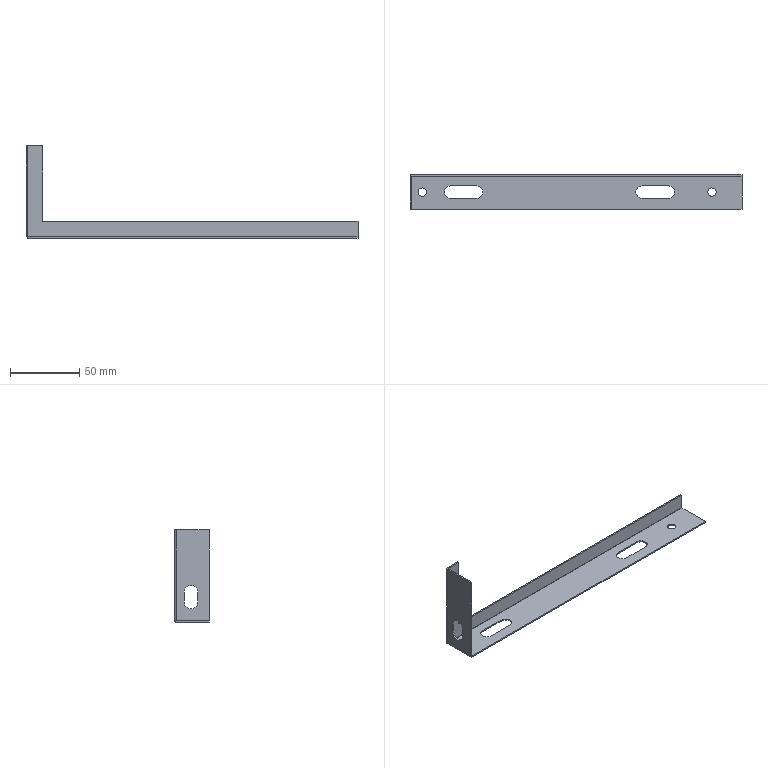Part | 1 solid | 40 faces | box 240 x 25 x 66.7 mm | volume 10129 mm3 | plane 26 | cylinder 14 | commonest cylinder face diameters 6 x4 9 x4 0.4 x2 2.4 x2 10 x2
STEP:
#1=CARTESIAN_POINT('',(97.7,-15.5,-0.2));
#2=VERTEX_POINT('',#1);
#3=CARTESIAN_POINT('',(97.7,-9.5,-0.2));
#4=VERTEX_POINT('',#3);
#5=CARTESIAN_POINT('',(97.7,-12.5,-0.2));
#6=DIRECTION('',(0.,0.,-1.));
#7=DIRECTION('',(0.,1.,0.));
#8=AXIS2_PLACEMENT_3D('',#5,#6,#7);
#9=CIRCLE('',#8,3.);
#10=EDGE_CURVE('',#2,#4,#9,.T.);
#11=ORIENTED_EDGE('',*,*,#10,.F.);
#12=CARTESIAN_POINT('',(97.7,-15.5,-1.2));
#13=VERTEX_POINT('',#12);
#14=CARTESIAN_POINT('',(97.7,-15.5,8.8));
#15=DIRECTION('',(0.,0.,-1.));
#16=VECTOR('',#15,1000.);
#17=LINE('',#14,#16);
#18=EDGE_CURVE('',#2,#13,#17,.T.);
#19=ORIENTED_EDGE('',*,*,#18,.T.);
#20=CARTESIAN_POINT('',(97.7,-9.5,-1.2));
#21=VERTEX_POINT('',#20);
#22=CARTESIAN_POINT('',(97.7,-12.5,-1.2));
#23=DIRECTION('',(0.,0.,-1.));
#24=DIRECTION('',(0.,1.,0.));
#25=AXIS2_PLACEMENT_3D('',#22,#23,#24);
#26=CIRCLE('',#25,3.);
#27=EDGE_CURVE('',#13,#21,#26,.T.);
#28=ORIENTED_EDGE('',*,*,#27,.T.);
#29=CARTESIAN_POINT('',(97.7,-9.5,8.8));
#30=DIRECTION('',(0.,0.,-1.));
#31=VECTOR('',#30,1000.);
#32=LINE('',#29,#31);
#33=EDGE_CURVE('',#4,#21,#32,.T.);
#34=ORIENTED_EDGE('',*,*,#33,.F.);
#35=EDGE_LOOP('',(#11,#19,#28,#34));
#36=FACE_OUTER_BOUND('',#35,.T.);
#37=CARTESIAN_POINT('',(97.7,-12.5,8.8));
#38=DIRECTION('',(0.,0.,-1.));
#39=DIRECTION('',(0.,1.,0.));
#40=AXIS2_PLACEMENT_3D('',#37,#38,#39);
#41=CYLINDRICAL_SURFACE('',#40,3.);
#42=ADVANCED_FACE('',(#36),#41,.F.);
#43=CARTESIAN_POINT('',(-111.8,-15.5,-0.2));
#44=VERTEX_POINT('',#43);
#45=CARTESIAN_POINT('',(-111.8,-9.5,-0.2));
#46=VERTEX_POINT('',#45);
#47=CARTESIAN_POINT('',(-111.8,-12.5,-0.2));
#48=DIRECTION('',(0.,0.,-1.));
#49=DIRECTION('',(0.,1.,0.));
#50=AXIS2_PLACEMENT_3D('',#47,#48,#49);
#51=CIRCLE('',#50,3.);
#52=EDGE_CURVE('',#44,#46,#51,.T.);
#53=ORIENTED_EDGE('',*,*,#52,.F.);
#54=CARTESIAN_POINT('',(-111.8,-15.5,-1.2));
#55=VERTEX_POINT('',#54);
#56=CARTESIAN_POINT('',(-111.8,-15.5,8.8));
#57=DIRECTION('',(0.,0.,-1.));
#58=VECTOR('',#57,1000.);
#59=LINE('',#56,#58);
#60=EDGE_CURVE('',#44,#55,#59,.T.);
#61=ORIENTED_EDGE('',*,*,#60,.T.);
#62=CARTESIAN_POINT('',(-111.8,-9.5,-1.2));
#63=VERTEX_POINT('',#62);
#64=CARTESIAN_POINT('',(-111.8,-12.5,-1.2));
#65=DIRECTION('',(0.,0.,-1.));
#66=DIRECTION('',(0.,1.,0.));
#67=AXIS2_PLACEMENT_3D('',#64,#65,#66);
#68=CIRCLE('',#67,3.);
#69=EDGE_CURVE('',#55,#63,#68,.T.);
#70=ORIENTED_EDGE('',*,*,#69,.T.);
#71=CARTESIAN_POINT('',(-111.8,-9.5,8.8));
#72=DIRECTION('',(0.,0.,-1.));
#73=VECTOR('',#72,1000.);
#74=LINE('',#71,#73);
#75=EDGE_CURVE('',#46,#63,#74,.T.);
#76=ORIENTED_EDGE('',*,*,#75,.F.);
#77=EDGE_LOOP('',(#53,#61,#70,#76));
#78=FACE_OUTER_BOUND('',#77,.T.);
#79=CARTESIAN_POINT('',(-111.8,-12.5,8.8));
#80=DIRECTION('',(0.,0.,-1.));
#81=DIRECTION('',(0.,1.,0.));
#82=AXIS2_PLACEMENT_3D('',#79,#80,#81);
#83=CYLINDRICAL_SURFACE('',#82,3.);
#84=ADVANCED_FACE('',(#78),#83,.F.);
#85=CARTESIAN_POINT('',(119.4,-1.,11.));
#86=VERTEX_POINT('',#85);
#87=CARTESIAN_POINT('',(-108.4,-1.,11.));
#88=VERTEX_POINT('',#87);
#89=CARTESIAN_POINT('',(-119.4,-1.,11.));
#90=DIRECTION('',(-1.,0.,0.));
#91=VECTOR('',#90,1000.);
#92=LINE('',#89,#91);
#93=EDGE_CURVE('',#86,#88,#92,.T.);
#94=ORIENTED_EDGE('',*,*,#93,.T.);
#95=CARTESIAN_POINT('',(-108.4,-1.,65.5));
#96=VERTEX_POINT('',#95);
#97=CARTESIAN_POINT('',(-108.4,-1.,65.5));
#98=DIRECTION('',(0.,0.,1.));
#99=VECTOR('',#98,1000.);
#100=LINE('',#97,#99);
#101=EDGE_CURVE('',#88,#96,#100,.T.);
#102=ORIENTED_EDGE('',*,*,#101,.T.);
#103=CARTESIAN_POINT('',(-119.4,-1.,65.5));
#104=VERTEX_POINT('',#103);
#105=CARTESIAN_POINT('',(-119.4,-1.,65.5));
#106=DIRECTION('',(1.,0.,0.));
#107=VECTOR('',#106,1000.);
#108=LINE('',#105,#107);
#109=EDGE_CURVE('',#104,#96,#108,.T.);
#110=ORIENTED_EDGE('',*,*,#109,.F.);
#111=CARTESIAN_POINT('',(-119.4,-1.,0.));
#112=VERTEX_POINT('',#111);
#113=CARTESIAN_POINT('',(-119.4,-1.,65.5));
#114=DIRECTION('',(0.,0.,-1.));
#115=VECTOR('',#114,1000.);
#116=LINE('',#113,#115);
#117=EDGE_CURVE('',#104,#112,#116,.T.);
#118=ORIENTED_EDGE('',*,*,#117,.T.);
#119=CARTESIAN_POINT('',(119.4,-1.,0.));
#120=VERTEX_POINT('',#119);
#121=CARTESIAN_POINT('',(-119.4,-1.,0.));
#122=DIRECTION('',(1.,0.,0.));
#123=VECTOR('',#122,1000.);
#124=LINE('',#121,#123);
#125=EDGE_CURVE('',#112,#120,#124,.T.);
#126=ORIENTED_EDGE('',*,*,#125,.T.);
#127=CARTESIAN_POINT('',(119.4,-1.,65.5));
#128=DIRECTION('',(0.,0.,-1.));
#129=VECTOR('',#128,1000.);
#130=LINE('',#127,#129);
#131=EDGE_CURVE('',#86,#120,#130,.T.);
#132=ORIENTED_EDGE('',*,*,#131,.F.);
#133=EDGE_LOOP('',(#94,#102,#110,#118,#126,#132));
#134=FACE_OUTER_BOUND('',#133,.T.);
#135=CARTESIAN_POINT('',(-119.4,-1.,65.5));
#136=DIRECTION('',(0.,1.,0.));
#137=DIRECTION('',(-1.,0.,0.));
#138=AXIS2_PLACEMENT_3D('',#135,#136,#137);
#139=PLANE('',#138);
#140=ADVANCED_FACE('',(#134),#139,.F.);
#141=CARTESIAN_POINT('',(119.4,0.,11.));
#142=VERTEX_POINT('',#141);
#143=CARTESIAN_POINT('',(119.4,-10.,11.));
#144=DIRECTION('',(0.,1.,0.));
#145=VECTOR('',#144,1000.);
#146=LINE('',#143,#145);
#147=EDGE_CURVE('',#86,#142,#146,.T.);
#148=ORIENTED_EDGE('',*,*,#147,.F.);
#149=ORIENTED_EDGE('',*,*,#131,.T.);
#150=CARTESIAN_POINT('',(119.4,0.,0.));
#151=VERTEX_POINT('',#150);
#152=CARTESIAN_POINT('',(119.4,0.,0.));
#153=DIRECTION('',(0.,-1.,0.));
#154=VECTOR('',#153,1000.);
#155=LINE('',#152,#154);
#156=EDGE_CURVE('',#151,#120,#155,.T.);
#157=ORIENTED_EDGE('',*,*,#156,.F.);
#158=CARTESIAN_POINT('',(119.4,0.,65.5));
#159=DIRECTION('',(0.,0.,-1.));
#160=VECTOR('',#159,1000.);
#161=LINE('',#158,#160);
#162=EDGE_CURVE('',#142,#151,#161,.T.);
#163=ORIENTED_EDGE('',*,*,#162,.F.);
#164=EDGE_LOOP('',(#148,#149,#157,#163));
#165=FACE_OUTER_BOUND('',#164,.T.);
#166=CARTESIAN_POINT('',(119.4,0.,65.5));
#167=DIRECTION('',(1.,0.,0.));
#168=DIRECTION('',(0.,0.,-1.));
#169=AXIS2_PLACEMENT_3D('',#166,#167,#168);
#170=PLANE('',#169);
#171=ADVANCED_FACE('',(#165),#170,.T.);
#172=CARTESIAN_POINT('',(-108.4,0.,11.));
#173=VERTEX_POINT('',#172);
#174=CARTESIAN_POINT('',(-108.4,0.,65.5));
#175=VERTEX_POINT('',#174);
#176=CARTESIAN_POINT('',(-108.4,0.,65.5));
#177=DIRECTION('',(0.,0.,1.));
#178=VECTOR('',#177,1000.);
#179=LINE('',#176,#178);
#180=EDGE_CURVE('',#173,#175,#179,.T.);
#181=ORIENTED_EDGE('',*,*,#180,.F.);
#182=CARTESIAN_POINT('',(119.4,0.,11.));
#183=DIRECTION('',(-1.,0.,0.));
#184=VECTOR('',#183,1000.);
#185=LINE('',#182,#184);
#186=EDGE_CURVE('',#142,#173,#185,.T.);
#187=ORIENTED_EDGE('',*,*,#186,.F.);
#188=ORIENTED_EDGE('',*,*,#162,.T.);
#189=CARTESIAN_POINT('',(-119.4,0.,0.));
#190=VERTEX_POINT('',#189);
#191=CARTESIAN_POINT('',(-119.4,0.,0.));
#192=DIRECTION('',(1.,0.,0.));
#193=VECTOR('',#192,1000.);
#194=LINE('',#191,#193);
#195=EDGE_CURVE('',#190,#151,#194,.T.);
#196=ORIENTED_EDGE('',*,*,#195,.F.);
#197=CARTESIAN_POINT('',(-119.4,0.,65.5));
#198=VERTEX_POINT('',#197);
#199=CARTESIAN_POINT('',(-119.4,0.,65.5));
#200=DIRECTION('',(0.,0.,-1.));
#201=VECTOR('',#200,1000.);
#202=LINE('',#199,#201);
#203=EDGE_CURVE('',#198,#190,#202,.T.);
#204=ORIENTED_EDGE('',*,*,#203,.F.);
#205=CARTESIAN_POINT('',(-119.4,0.,65.5));
#206=DIRECTION('',(1.,0.,0.));
#207=VECTOR('',#206,1000.);
#208=LINE('',#205,#207);
#209=EDGE_CURVE('',#198,#175,#208,.T.);
#210=ORIENTED_EDGE('',*,*,#209,.T.);
#211=EDGE_LOOP('',(#181,#187,#188,#196,#204,#210));
#212=FACE_OUTER_BOUND('',#211,.T.);
#213=CARTESIAN_POINT('',(-119.4,0.,65.5));
#214=DIRECTION('',(0.,1.,0.));
#215=DIRECTION('',(-1.,0.,0.));
#216=AXIS2_PLACEMENT_3D('',#213,#214,#215);
#217=PLANE('',#216);
#218=ADVANCED_FACE('',(#212),#217,.T.);
#219=ORIENTED_EDGE('',*,*,#109,.T.);
#220=CARTESIAN_POINT('',(-108.4,0.,65.5));
#221=DIRECTION('',(0.,1.,0.));
#222=VECTOR('',#221,1000.);
#223=LINE('',#220,#222);
#224=EDGE_CURVE('',#96,#175,#223,.T.);
#225=ORIENTED_EDGE('',*,*,#224,.T.);
#226=ORIENTED_EDGE('',*,*,#209,.F.);
#227=CARTESIAN_POINT('',(-119.4,-1.,65.5));
#228=DIRECTION('',(0.,1.,0.));
#229=VECTOR('',#228,1000.);
#230=LINE('',#227,#229);
#231=EDGE_CURVE('',#104,#198,#230,.T.);
#232=ORIENTED_EDGE('',*,*,#231,.F.);
#233=EDGE_LOOP('',(#219,#225,#226,#232));
#234=FACE_OUTER_BOUND('',#233,.T.);
#235=CARTESIAN_POINT('',(0.,0.,65.5));
#236=DIRECTION('',(0.,0.,-1.));
#237=DIRECTION('',(-1.,0.,0.));
#238=AXIS2_PLACEMENT_3D('',#235,#236,#237);
#239=PLANE('',#238);
#240=ADVANCED_FACE('',(#234),#239,.F.);
#241=ORIENTED_EDGE('',*,*,#147,.T.);
#242=ORIENTED_EDGE('',*,*,#186,.T.);
#243=CARTESIAN_POINT('',(-108.4,-10.,11.));
#244=DIRECTION('',(0.,1.,0.));
#245=VECTOR('',#244,1000.);
#246=LINE('',#243,#245);
#247=EDGE_CURVE('',#88,#173,#246,.T.);
#248=ORIENTED_EDGE('',*,*,#247,.F.);
#249=ORIENTED_EDGE('',*,*,#93,.F.);
#250=EDGE_LOOP('',(#241,#242,#248,#249));
#251=FACE_OUTER_BOUND('',#250,.T.);
#252=CARTESIAN_POINT('',(119.4,-10.,11.));
#253=DIRECTION('',(0.,0.,-1.));
#254=DIRECTION('',(-1.,0.,0.));
#255=AXIS2_PLACEMENT_3D('',#252,#253,#254);
#256=PLANE('',#255);
#257=ADVANCED_FACE('',(#251),#256,.F.);
#258=ORIENTED_EDGE('',*,*,#247,.T.);
#259=ORIENTED_EDGE('',*,*,#180,.T.);
#260=ORIENTED_EDGE('',*,*,#224,.F.);
#261=ORIENTED_EDGE('',*,*,#101,.F.);
#262=EDGE_LOOP('',(#258,#259,#260,#261));
#263=FACE_OUTER_BOUND('',#262,.T.);
#264=CARTESIAN_POINT('',(-108.4,-10.,65.5));
#265=DIRECTION('',(-1.,0.,0.));
#266=DIRECTION('',(0.,0.,1.));
#267=AXIS2_PLACEMENT_3D('',#264,#265,#266);
#268=PLANE('',#267);
#269=ADVANCED_FACE('',(#263),#268,.F.);
#270=CARTESIAN_POINT('',(-119.4,-1.2,-0.2));
#271=VERTEX_POINT('',#270);
#272=CARTESIAN_POINT('',(-119.4,-1.2,-1.2));
#273=VERTEX_POINT('',#272);
#274=CARTESIAN_POINT('',(-119.4,-1.2,-1.2));
#275=DIRECTION('',(0.,0.,-1.));
#276=VECTOR('',#275,1000.);
#277=LINE('',#274,#276);
#278=EDGE_CURVE('',#271,#273,#277,.T.);
#279=ORIENTED_EDGE('',*,*,#278,.F.);
#280=CARTESIAN_POINT('',(-119.4,-1.2,0.));
#281=DIRECTION('',(-1.,0.,0.));
#282=DIRECTION('',(0.,1.,0.));
#283=AXIS2_PLACEMENT_3D('',#280,#281,#282);
#284=CIRCLE('',#283,0.2);
#285=EDGE_CURVE('',#112,#271,#284,.T.);
#286=ORIENTED_EDGE('',*,*,#285,.F.);
#287=CARTESIAN_POINT('',(-119.4,-1.,0.));
#288=DIRECTION('',(0.,1.,0.));
#289=VECTOR('',#288,1000.);
#290=LINE('',#287,#289);
#291=EDGE_CURVE('',#112,#190,#290,.T.);
#292=ORIENTED_EDGE('',*,*,#291,.T.);
#293=CARTESIAN_POINT('',(-119.4,-1.2,0.));
#294=DIRECTION('',(-1.,0.,0.));
#295=DIRECTION('',(0.,1.,0.));
#296=AXIS2_PLACEMENT_3D('',#293,#294,#295);
#297=CIRCLE('',#296,1.2);
#298=EDGE_CURVE('',#190,#273,#297,.T.);
#299=ORIENTED_EDGE('',*,*,#298,.T.);
#300=EDGE_LOOP('',(#279,#286,#292,#299));
#301=FACE_OUTER_BOUND('',#300,.T.);
#302=CARTESIAN_POINT('',(-119.4,-1.2,0.));
#303=DIRECTION('',(-1.,0.,0.));
#304=DIRECTION('',(0.,-1.,0.));
#305=AXIS2_PLACEMENT_3D('',#302,#303,#304);
#306=PLANE('',#305);
#307=ADVANCED_FACE('',(#301),#306,.T.);
#308=CARTESIAN_POINT('',(119.4,-1.2,-0.2));
#309=VERTEX_POINT('',#308);
#310=CARTESIAN_POINT('',(119.4,-1.2,0.));
#311=DIRECTION('',(1.,0.,0.));
#312=DIRECTION('',(0.,1.,0.));
#313=AXIS2_PLACEMENT_3D('',#310,#311,#312);
#314=CIRCLE('',#313,0.2);
#315=EDGE_CURVE('',#309,#120,#314,.T.);
#316=ORIENTED_EDGE('',*,*,#315,.F.);
#317=CARTESIAN_POINT('',(119.4,-1.2,-1.2));
#318=VERTEX_POINT('',#317);
#319=CARTESIAN_POINT('',(119.4,-1.2,-0.2));
#320=DIRECTION('',(0.,0.,-1.));
#321=VECTOR('',#320,1000.);
#322=LINE('',#319,#321);
#323=EDGE_CURVE('',#309,#318,#322,.T.);
#324=ORIENTED_EDGE('',*,*,#323,.T.);
#325=CARTESIAN_POINT('',(119.4,-1.2,0.));
#326=DIRECTION('',(1.,0.,0.));
#327=DIRECTION('',(0.,1.,0.));
#328=AXIS2_PLACEMENT_3D('',#325,#326,#327);
#329=CIRCLE('',#328,1.2);
#330=EDGE_CURVE('',#318,#151,#329,.T.);
#331=ORIENTED_EDGE('',*,*,#330,.T.);
#332=ORIENTED_EDGE('',*,*,#156,.T.);
#333=EDGE_LOOP('',(#316,#324,#331,#332));
#334=FACE_OUTER_BOUND('',#333,.T.);
#335=CARTESIAN_POINT('',(119.4,-1.2,0.));
#336=DIRECTION('',(-1.,0.,0.));
#337=DIRECTION('',(0.,-1.,0.));
#338=AXIS2_PLACEMENT_3D('',#335,#336,#337);
#339=PLANE('',#338);
#340=ADVANCED_FACE('',(#334),#339,.F.);
#341=ORIENTED_EDGE('',*,*,#195,.T.);
#342=ORIENTED_EDGE('',*,*,#330,.F.);
#343=CARTESIAN_POINT('',(0.,-1.2,-1.2));
#344=DIRECTION('',(1.,0.,0.));
#345=VECTOR('',#344,1000.);
#346=LINE('',#343,#345);
#347=EDGE_CURVE('',#273,#318,#346,.T.);
#348=ORIENTED_EDGE('',*,*,#347,.F.);
#349=ORIENTED_EDGE('',*,*,#298,.F.);
#350=EDGE_LOOP('',(#341,#342,#348,#349));
#351=FACE_OUTER_BOUND('',#350,.T.);
#352=CARTESIAN_POINT('',(119.4,-1.2,0.));
#353=DIRECTION('',(1.,0.,0.));
#354=DIRECTION('',(0.,0.,-1.));
#355=AXIS2_PLACEMENT_3D('',#352,#353,#354);
#356=CYLINDRICAL_SURFACE('',#355,1.2);
#357=ADVANCED_FACE('',(#351),#356,.T.);
#358=ORIENTED_EDGE('',*,*,#125,.F.);
#359=ORIENTED_EDGE('',*,*,#285,.T.);
#360=CARTESIAN_POINT('',(-119.4,-1.2,-0.2));
#361=DIRECTION('',(1.,0.,0.));
#362=VECTOR('',#361,1000.);
#363=LINE('',#360,#362);
#364=EDGE_CURVE('',#271,#309,#363,.T.);
#365=ORIENTED_EDGE('',*,*,#364,.T.);
#366=ORIENTED_EDGE('',*,*,#315,.T.);
#367=EDGE_LOOP('',(#358,#359,#365,#366));
#368=FACE_OUTER_BOUND('',#367,.T.);
#369=CARTESIAN_POINT('',(119.4,-1.2,0.));
#370=DIRECTION('',(1.,0.,0.));
#371=DIRECTION('',(0.,0.,-1.));
#372=AXIS2_PLACEMENT_3D('',#369,#370,#371);
#373=CYLINDRICAL_SURFACE('',#372,0.2);
#374=ADVANCED_FACE('',(#368),#373,.F.);
#375=CARTESIAN_POINT('',(119.4,-25.,-1.2));
#376=VERTEX_POINT('',#375);
#377=CARTESIAN_POINT('',(119.4,-1.,-1.2));
#378=DIRECTION('',(0.,1.,0.));
#379=VECTOR('',#378,1000.);
#380=LINE('',#377,#379);
#381=EDGE_CURVE('',#376,#318,#380,.T.);
#382=ORIENTED_EDGE('',*,*,#381,.T.);
#383=ORIENTED_EDGE('',*,*,#323,.F.);
#384=CARTESIAN_POINT('',(119.4,-25.,-0.2));
#385=VERTEX_POINT('',#384);
#386=CARTESIAN_POINT('',(119.4,0.,-0.2));
#387=DIRECTION('',(0.,1.,0.));
#388=VECTOR('',#387,1000.);
#389=LINE('',#386,#388);
#390=EDGE_CURVE('',#385,#309,#389,.T.);
#391=ORIENTED_EDGE('',*,*,#390,.F.);
#392=CARTESIAN_POINT('',(119.4,-25.,-1.2));
#393=DIRECTION('',(0.,0.,1.));
#394=VECTOR('',#393,1000.);
#395=LINE('',#392,#394);
#396=EDGE_CURVE('',#376,#385,#395,.T.);
#397=ORIENTED_EDGE('',*,*,#396,.F.);
#398=EDGE_LOOP('',(#382,#383,#391,#397));
#399=FACE_OUTER_BOUND('',#398,.T.);
#400=CARTESIAN_POINT('',(119.4,-1.,-1.2));
#401=DIRECTION('',(1.,0.,0.));
#402=DIRECTION('',(0.,0.,-1.));
#403=AXIS2_PLACEMENT_3D('',#400,#401,#402);
#404=PLANE('',#403);
#405=ADVANCED_FACE('',(#399),#404,.T.);
#406=CARTESIAN_POINT('',(-119.4,-25.,-0.2));
#407=VERTEX_POINT('',#406);
#408=CARTESIAN_POINT('',(-119.4,0.,-0.2));
#409=DIRECTION('',(0.,-1.,0.));
#410=VECTOR('',#409,1000.);
#411=LINE('',#408,#410);
#412=EDGE_CURVE('',#271,#407,#411,.T.);
#413=ORIENTED_EDGE('',*,*,#412,.F.);
#414=ORIENTED_EDGE('',*,*,#278,.T.);
#415=CARTESIAN_POINT('',(-119.4,-25.,-1.2));
#416=VERTEX_POINT('',#415);
#417=CARTESIAN_POINT('',(-119.4,-25.,-1.2));
#418=DIRECTION('',(0.,-1.,0.));
#419=VECTOR('',#418,1000.);
#420=LINE('',#417,#419);
#421=EDGE_CURVE('',#273,#416,#420,.T.);
#422=ORIENTED_EDGE('',*,*,#421,.T.);
#423=CARTESIAN_POINT('',(-119.4,-25.,-1.2));
#424=DIRECTION('',(0.,0.,1.));
#425=VECTOR('',#424,1000.);
#426=LINE('',#423,#425);
#427=EDGE_CURVE('',#416,#407,#426,.T.);
#428=ORIENTED_EDGE('',*,*,#427,.T.);
#429=EDGE_LOOP('',(#413,#414,#422,#428));
#430=FACE_OUTER_BOUND('',#429,.T.);
#431=CARTESIAN_POINT('',(-119.4,-25.,-1.2));
#432=DIRECTION('',(-1.,0.,0.));
#433=DIRECTION('',(0.,0.,1.));
#434=AXIS2_PLACEMENT_3D('',#431,#432,#433);
#435=PLANE('',#434);
#436=ADVANCED_FACE('',(#430),#435,.T.);
#437=CARTESIAN_POINT('',(97.7,-12.5,-1.2));
#438=DIRECTION('',(0.,0.,-1.));
#439=DIRECTION('',(0.,1.,0.));
#440=AXIS2_PLACEMENT_3D('',#437,#438,#439);
#441=CIRCLE('',#440,3.);
#442=EDGE_CURVE('',#21,#13,#441,.T.);
#443=ORIENTED_EDGE('',*,*,#442,.F.);
#444=ORIENTED_EDGE('',*,*,#27,.F.);
#445=EDGE_LOOP('',(#443,#444));
#446=FACE_BOUND('',#445,.T.);
#447=CARTESIAN_POINT('',(-111.8,-12.5,-1.2));
#448=DIRECTION('',(0.,0.,-1.));
#449=DIRECTION('',(0.,1.,0.));
#450=AXIS2_PLACEMENT_3D('',#447,#448,#449);
#451=CIRCLE('',#450,3.);
#452=EDGE_CURVE('',#63,#55,#451,.T.);
#453=ORIENTED_EDGE('',*,*,#452,.F.);
#454=ORIENTED_EDGE('',*,*,#69,.F.);
#455=EDGE_LOOP('',(#453,#454));
#456=FACE_BOUND('',#455,.T.);
#457=CARTESIAN_POINT('',(47.2,-17.,-1.2));
#458=VERTEX_POINT('',#457);
#459=CARTESIAN_POINT('',(47.2,-8.,-1.2));
#460=VERTEX_POINT('',#459);
#461=CARTESIAN_POINT('',(47.2,-12.5,-1.2));
#462=DIRECTION('',(0.,0.,-1.));
#463=DIRECTION('',(0.,1.,0.));
#464=AXIS2_PLACEMENT_3D('',#461,#462,#463);
#465=CIRCLE('',#464,4.5);
#466=EDGE_CURVE('',#458,#460,#465,.T.);
#467=ORIENTED_EDGE('',*,*,#466,.F.);
#468=CARTESIAN_POINT('',(66.2,-17.,-1.2));
#469=VERTEX_POINT('',#468);
#470=CARTESIAN_POINT('',(47.2,-17.,-1.2));
#471=DIRECTION('',(-1.,0.,0.));
#472=VECTOR('',#471,1000.);
#473=LINE('',#470,#472);
#474=EDGE_CURVE('',#469,#458,#473,.T.);
#475=ORIENTED_EDGE('',*,*,#474,.F.);
#476=CARTESIAN_POINT('',(66.2,-8.,-1.2));
#477=VERTEX_POINT('',#476);
#478=CARTESIAN_POINT('',(66.2,-12.5,-1.2));
#479=DIRECTION('',(0.,0.,-1.));
#480=DIRECTION('',(0.,1.,0.));
#481=AXIS2_PLACEMENT_3D('',#478,#479,#480);
#482=CIRCLE('',#481,4.5);
#483=EDGE_CURVE('',#477,#469,#482,.T.);
#484=ORIENTED_EDGE('',*,*,#483,.F.);
#485=CARTESIAN_POINT('',(47.2,-8.,-1.2));
#486=DIRECTION('',(1.,0.,0.));
#487=VECTOR('',#486,1000.);
#488=LINE('',#485,#487);
#489=EDGE_CURVE('',#460,#477,#488,.T.);
#490=ORIENTED_EDGE('',*,*,#489,.F.);
#491=EDGE_LOOP('',(#467,#475,#484,#490));
#492=FACE_BOUND('',#491,.T.);
#493=CARTESIAN_POINT('',(-91.3,-17.,-1.2));
#494=VERTEX_POINT('',#493);
#495=CARTESIAN_POINT('',(-91.3,-8.,-1.2));
#496=VERTEX_POINT('',#495);
#497=CARTESIAN_POINT('',(-91.3,-12.5,-1.2));
#498=DIRECTION('',(0.,0.,-1.));
#499=DIRECTION('',(0.,1.,0.));
#500=AXIS2_PLACEMENT_3D('',#497,#498,#499);
#501=CIRCLE('',#500,4.5);
#502=EDGE_CURVE('',#494,#496,#501,.T.);
#503=ORIENTED_EDGE('',*,*,#502,.F.);
#504=CARTESIAN_POINT('',(-72.3,-17.,-1.2));
#505=VERTEX_POINT('',#504);
#506=CARTESIAN_POINT('',(-91.3,-17.,-1.2));
#507=DIRECTION('',(-1.,0.,0.));
#508=VECTOR('',#507,1000.);
#509=LINE('',#506,#508);
#510=EDGE_CURVE('',#505,#494,#509,.T.);
#511=ORIENTED_EDGE('',*,*,#510,.F.);
#512=CARTESIAN_POINT('',(-72.3,-8.,-1.2));
#513=VERTEX_POINT('',#512);
#514=CARTESIAN_POINT('',(-72.3,-12.5,-1.2));
#515=DIRECTION('',(0.,0.,-1.));
#516=DIRECTION('',(0.,1.,0.));
#517=AXIS2_PLACEMENT_3D('',#514,#515,#516);
#518=CIRCLE('',#517,4.5);
#519=EDGE_CURVE('',#513,#505,#518,.T.);
#520=ORIENTED_EDGE('',*,*,#519,.F.);
#521=CARTESIAN_POINT('',(-91.3,-8.,-1.2));
#522=DIRECTION('',(1.,0.,0.));
#523=VECTOR('',#522,1000.);
#524=LINE('',#521,#523);
#525=EDGE_CURVE('',#496,#513,#524,.T.);
#526=ORIENTED_EDGE('',*,*,#525,.F.);
#527=EDGE_LOOP('',(#503,#511,#520,#526));
#528=FACE_BOUND('',#527,.T.);
#529=ORIENTED_EDGE('',*,*,#421,.F.);
#530=ORIENTED_EDGE('',*,*,#347,.T.);
#531=ORIENTED_EDGE('',*,*,#381,.F.);
#532=CARTESIAN_POINT('',(119.4,-25.,-1.2));
#533=DIRECTION('',(1.,0.,0.));
#534=VECTOR('',#533,1000.);
#535=LINE('',#532,#534);
#536=EDGE_CURVE('',#416,#376,#535,.T.);
#537=ORIENTED_EDGE('',*,*,#536,.F.);
#538=EDGE_LOOP('',(#529,#530,#531,#537));
#539=FACE_OUTER_BOUND('',#538,.T.);
#540=CARTESIAN_POINT('',(0.,0.,-1.2));
#541=DIRECTION('',(0.,0.,-1.));
#542=DIRECTION('',(0.,1.,0.));
#543=AXIS2_PLACEMENT_3D('',#540,#541,#542);
#544=PLANE('',#543);
#545=ADVANCED_FACE('',(#446,#456,#492,#528,#539),#544,.T.);
#546=CARTESIAN_POINT('',(97.7,-12.5,-0.2));
#547=DIRECTION('',(0.,0.,-1.));
#548=DIRECTION('',(0.,1.,0.));
#549=AXIS2_PLACEMENT_3D('',#546,#547,#548);
#550=CIRCLE('',#549,3.);
#551=EDGE_CURVE('',#4,#2,#550,.T.);
#552=ORIENTED_EDGE('',*,*,#551,.T.);
#553=ORIENTED_EDGE('',*,*,#10,.T.);
#554=EDGE_LOOP('',(#552,#553));
#555=FACE_BOUND('',#554,.T.);
#556=CARTESIAN_POINT('',(-111.8,-12.5,-0.2));
#557=DIRECTION('',(0.,0.,-1.));
#558=DIRECTION('',(0.,1.,0.));
#559=AXIS2_PLACEMENT_3D('',#556,#557,#558);
#560=CIRCLE('',#559,3.);
#561=EDGE_CURVE('',#46,#44,#560,.T.);
#562=ORIENTED_EDGE('',*,*,#561,.T.);
#563=ORIENTED_EDGE('',*,*,#52,.T.);
#564=EDGE_LOOP('',(#562,#563));
#565=FACE_BOUND('',#564,.T.);
#566=CARTESIAN_POINT('',(66.2,-17.,-0.2));
#567=VERTEX_POINT('',#566);
#568=CARTESIAN_POINT('',(47.2,-17.,-0.2));
#569=VERTEX_POINT('',#568);
#570=CARTESIAN_POINT('',(0.,-17.,-0.2));
#571=DIRECTION('',(-1.,0.,0.));
#572=VECTOR('',#571,1000.);
#573=LINE('',#570,#572);
#574=EDGE_CURVE('',#567,#569,#573,.T.);
#575=ORIENTED_EDGE('',*,*,#574,.T.);
#576=CARTESIAN_POINT('',(47.2,-8.,-0.2));
#577=VERTEX_POINT('',#576);
#578=CARTESIAN_POINT('',(47.2,-12.5,-0.2));
#579=DIRECTION('',(0.,0.,-1.));
#580=DIRECTION('',(0.,1.,0.));
#581=AXIS2_PLACEMENT_3D('',#578,#579,#580);
#582=CIRCLE('',#581,4.5);
#583=EDGE_CURVE('',#569,#577,#582,.T.);
#584=ORIENTED_EDGE('',*,*,#583,.T.);
#585=CARTESIAN_POINT('',(66.2,-8.,-0.2));
#586=VERTEX_POINT('',#585);
#587=CARTESIAN_POINT('',(0.,-8.,-0.2));
#588=DIRECTION('',(1.,0.,0.));
#589=VECTOR('',#588,1000.);
#590=LINE('',#587,#589);
#591=EDGE_CURVE('',#577,#586,#590,.T.);
#592=ORIENTED_EDGE('',*,*,#591,.T.);
#593=CARTESIAN_POINT('',(66.2,-12.5,-0.2));
#594=DIRECTION('',(0.,0.,-1.));
#595=DIRECTION('',(0.,1.,0.));
#596=AXIS2_PLACEMENT_3D('',#593,#594,#595);
#597=CIRCLE('',#596,4.5);
#598=EDGE_CURVE('',#586,#567,#597,.T.);
#599=ORIENTED_EDGE('',*,*,#598,.T.);
#600=EDGE_LOOP('',(#575,#584,#592,#599));
#601=FACE_BOUND('',#600,.T.);
#602=CARTESIAN_POINT('',(-72.3,-17.,-0.2));
#603=VERTEX_POINT('',#602);
#604=CARTESIAN_POINT('',(-91.3,-17.,-0.2));
#605=VERTEX_POINT('',#604);
#606=CARTESIAN_POINT('',(0.,-17.,-0.2));
#607=DIRECTION('',(-1.,0.,0.));
#608=VECTOR('',#607,1000.);
#609=LINE('',#606,#608);
#610=EDGE_CURVE('',#603,#605,#609,.T.);
#611=ORIENTED_EDGE('',*,*,#610,.T.);
#612=CARTESIAN_POINT('',(-91.3,-8.,-0.2));
#613=VERTEX_POINT('',#612);
#614=CARTESIAN_POINT('',(-91.3,-12.5,-0.2));
#615=DIRECTION('',(0.,0.,-1.));
#616=DIRECTION('',(0.,1.,0.));
#617=AXIS2_PLACEMENT_3D('',#614,#615,#616);
#618=CIRCLE('',#617,4.5);
#619=EDGE_CURVE('',#605,#613,#618,.T.);
#620=ORIENTED_EDGE('',*,*,#619,.T.);
#621=CARTESIAN_POINT('',(-72.3,-8.,-0.2));
#622=VERTEX_POINT('',#621);
#623=CARTESIAN_POINT('',(0.,-8.,-0.2));
#624=DIRECTION('',(1.,0.,0.));
#625=VECTOR('',#624,1000.);
#626=LINE('',#623,#625);
#627=EDGE_CURVE('',#613,#622,#626,.T.);
#628=ORIENTED_EDGE('',*,*,#627,.T.);
#629=CARTESIAN_POINT('',(-72.3,-12.5,-0.2));
#630=DIRECTION('',(0.,0.,-1.));
#631=DIRECTION('',(0.,1.,0.));
#632=AXIS2_PLACEMENT_3D('',#629,#630,#631);
#633=CIRCLE('',#632,4.5);
#634=EDGE_CURVE('',#622,#603,#633,.T.);
#635=ORIENTED_EDGE('',*,*,#634,.T.);
#636=EDGE_LOOP('',(#611,#620,#628,#635));
#637=FACE_BOUND('',#636,.T.);
#638=ORIENTED_EDGE('',*,*,#364,.F.);
#639=ORIENTED_EDGE('',*,*,#412,.T.);
#640=CARTESIAN_POINT('',(0.,-25.,-0.2));
#641=DIRECTION('',(1.,0.,0.));
#642=VECTOR('',#641,1000.);
#643=LINE('',#640,#642);
#644=EDGE_CURVE('',#407,#385,#643,.T.);
#645=ORIENTED_EDGE('',*,*,#644,.T.);
#646=ORIENTED_EDGE('',*,*,#390,.T.);
#647=EDGE_LOOP('',(#638,#639,#645,#646));
#648=FACE_OUTER_BOUND('',#647,.T.);
#649=CARTESIAN_POINT('',(0.,0.,-0.2));
#650=DIRECTION('',(0.,0.,-1.));
#651=DIRECTION('',(0.,1.,0.));
#652=AXIS2_PLACEMENT_3D('',#649,#650,#651);
#653=PLANE('',#652);
#654=ADVANCED_FACE('',(#555,#565,#601,#637,#648),#653,.F.);
#655=ORIENTED_EDGE('',*,*,#644,.F.);
#656=ORIENTED_EDGE('',*,*,#427,.F.);
#657=ORIENTED_EDGE('',*,*,#536,.T.);
#658=ORIENTED_EDGE('',*,*,#396,.T.);
#659=EDGE_LOOP('',(#655,#656,#657,#658));
#660=FACE_OUTER_BOUND('',#659,.T.);
#661=CARTESIAN_POINT('',(119.4,-25.,-1.2));
#662=DIRECTION('',(0.,-1.,0.));
#663=DIRECTION('',(0.,0.,-1.));
#664=AXIS2_PLACEMENT_3D('',#661,#662,#663);
#665=PLANE('',#664);
#666=ADVANCED_FACE('',(#660),#665,.T.);
#667=CARTESIAN_POINT('',(-119.6,-1.2,65.5));
#668=VERTEX_POINT('',#667);
#669=CARTESIAN_POINT('',(-120.6,-1.2,65.5));
#670=VERTEX_POINT('',#669);
#671=CARTESIAN_POINT('',(-120.6,-1.2,65.5));
#672=DIRECTION('',(-1.,0.,0.));
#673=VECTOR('',#672,1000.);
#674=LINE('',#671,#673);
#675=EDGE_CURVE('',#668,#670,#674,.T.);
#676=ORIENTED_EDGE('',*,*,#675,.F.);
#677=CARTESIAN_POINT('',(-119.4,-1.2,65.5));
#678=DIRECTION('',(0.,0.,1.));
#679=DIRECTION('',(-1.,0.,0.));
#680=AXIS2_PLACEMENT_3D('',#677,#678,#679);
#681=CIRCLE('',#680,0.2);
#682=EDGE_CURVE('',#104,#668,#681,.T.);
#683=ORIENTED_EDGE('',*,*,#682,.F.);
#684=ORIENTED_EDGE('',*,*,#231,.T.);
#685=CARTESIAN_POINT('',(-119.4,-1.2,65.5));
#686=DIRECTION('',(0.,0.,1.));
#687=DIRECTION('',(-1.,0.,0.));
#688=AXIS2_PLACEMENT_3D('',#685,#686,#687);
#689=CIRCLE('',#688,1.2);
#690=EDGE_CURVE('',#198,#670,#689,.T.);
#691=ORIENTED_EDGE('',*,*,#690,.T.);
#692=EDGE_LOOP('',(#676,#683,#684,#691));
#693=FACE_OUTER_BOUND('',#692,.T.);
#694=CARTESIAN_POINT('',(-119.4,-1.2,65.5));
#695=DIRECTION('',(0.,0.,1.));
#696=DIRECTION('',(1.,0.,0.));
#697=AXIS2_PLACEMENT_3D('',#694,#695,#696);
#698=PLANE('',#697);
#699=ADVANCED_FACE('',(#693),#698,.T.);
#700=CARTESIAN_POINT('',(-119.6,-1.2,0.));
#701=VERTEX_POINT('',#700);
#702=CARTESIAN_POINT('',(-119.4,-1.2,0.));
#703=DIRECTION('',(0.,0.,-1.));
#704=DIRECTION('',(-1.,0.,0.));
#705=AXIS2_PLACEMENT_3D('',#702,#703,#704);
#706=CIRCLE('',#705,0.2);
#707=EDGE_CURVE('',#701,#112,#706,.T.);
#708=ORIENTED_EDGE('',*,*,#707,.F.);
#709=CARTESIAN_POINT('',(-120.6,-1.2,0.));
#710=VERTEX_POINT('',#709);
#711=CARTESIAN_POINT('',(-119.6,-1.2,0.));
#712=DIRECTION('',(-1.,0.,0.));
#713=VECTOR('',#712,1000.);
#714=LINE('',#711,#713);
#715=EDGE_CURVE('',#701,#710,#714,.T.);
#716=ORIENTED_EDGE('',*,*,#715,.T.);
#717=CARTESIAN_POINT('',(-119.4,-1.2,0.));
#718=DIRECTION('',(0.,0.,-1.));
#719=DIRECTION('',(-1.,0.,0.));
#720=AXIS2_PLACEMENT_3D('',#717,#718,#719);
#721=CIRCLE('',#720,1.2);
#722=EDGE_CURVE('',#710,#190,#721,.T.);
#723=ORIENTED_EDGE('',*,*,#722,.T.);
#724=ORIENTED_EDGE('',*,*,#291,.F.);
#725=EDGE_LOOP('',(#708,#716,#723,#724));
#726=FACE_OUTER_BOUND('',#725,.T.);
#727=CARTESIAN_POINT('',(-119.4,-1.2,0.));
#728=DIRECTION('',(0.,0.,1.));
#729=DIRECTION('',(1.,0.,0.));
#730=AXIS2_PLACEMENT_3D('',#727,#728,#729);
#731=PLANE('',#730);
#732=ADVANCED_FACE('',(#726),#731,.F.);
#733=ORIENTED_EDGE('',*,*,#203,.T.);
#734=ORIENTED_EDGE('',*,*,#722,.F.);
#735=CARTESIAN_POINT('',(-120.6,-1.2,0.));
#736=DIRECTION('',(0.,0.,-1.));
#737=VECTOR('',#736,1000.);
#738=LINE('',#735,#737);
#739=EDGE_CURVE('',#670,#710,#738,.T.);
#740=ORIENTED_EDGE('',*,*,#739,.F.);
#741=ORIENTED_EDGE('',*,*,#690,.F.);
#742=EDGE_LOOP('',(#733,#734,#740,#741));
#743=FACE_OUTER_BOUND('',#742,.T.);
#744=CARTESIAN_POINT('',(-119.4,-1.2,0.));
#745=DIRECTION('',(0.,0.,-1.));
#746=DIRECTION('',(-1.,0.,0.));
#747=AXIS2_PLACEMENT_3D('',#744,#745,#746);
#748=CYLINDRICAL_SURFACE('',#747,1.2);
#749=ADVANCED_FACE('',(#743),#748,.T.);
#750=ORIENTED_EDGE('',*,*,#117,.F.);
#751=ORIENTED_EDGE('',*,*,#682,.T.);
#752=CARTESIAN_POINT('',(-119.6,-1.2,65.5));
#753=DIRECTION('',(0.,0.,-1.));
#754=VECTOR('',#753,1000.);
#755=LINE('',#752,#754);
#756=EDGE_CURVE('',#668,#701,#755,.T.);
#757=ORIENTED_EDGE('',*,*,#756,.T.);
#758=ORIENTED_EDGE('',*,*,#707,.T.);
#759=EDGE_LOOP('',(#750,#751,#757,#758));
#760=FACE_OUTER_BOUND('',#759,.T.);
#761=CARTESIAN_POINT('',(-119.4,-1.2,0.));
#762=DIRECTION('',(0.,0.,-1.));
#763=DIRECTION('',(-1.,0.,0.));
#764=AXIS2_PLACEMENT_3D('',#761,#762,#763);
#765=CYLINDRICAL_SURFACE('',#764,0.2);
#766=ADVANCED_FACE('',(#760),#765,.F.);
#767=CARTESIAN_POINT('',(-120.6,-25.,0.));
#768=VERTEX_POINT('',#767);
#769=CARTESIAN_POINT('',(-120.6,-1.,0.));
#770=DIRECTION('',(0.,1.,0.));
#771=VECTOR('',#770,1000.);
#772=LINE('',#769,#771);
#773=EDGE_CURVE('',#768,#710,#772,.T.);
#774=ORIENTED_EDGE('',*,*,#773,.T.);
#775=ORIENTED_EDGE('',*,*,#715,.F.);
#776=CARTESIAN_POINT('',(-119.6,-25.,0.));
#777=VERTEX_POINT('',#776);
#778=CARTESIAN_POINT('',(-119.6,0.,0.));
#779=DIRECTION('',(0.,1.,0.));
#780=VECTOR('',#779,1000.);
#781=LINE('',#778,#780);
#782=EDGE_CURVE('',#777,#701,#781,.T.);
#783=ORIENTED_EDGE('',*,*,#782,.F.);
#784=CARTESIAN_POINT('',(-120.6,-25.,0.));
#785=DIRECTION('',(1.,0.,0.));
#786=VECTOR('',#785,1000.);
#787=LINE('',#784,#786);
#788=EDGE_CURVE('',#768,#777,#787,.T.);
#789=ORIENTED_EDGE('',*,*,#788,.F.);
#790=EDGE_LOOP('',(#774,#775,#783,#789));
#791=FACE_OUTER_BOUND('',#790,.T.);
#792=CARTESIAN_POINT('',(-120.6,-1.,0.));
#793=DIRECTION('',(0.,0.,-1.));
#794=DIRECTION('',(-1.,0.,0.));
#795=AXIS2_PLACEMENT_3D('',#792,#793,#794);
#796=PLANE('',#795);
#797=ADVANCED_FACE('',(#791),#796,.T.);
#798=CARTESIAN_POINT('',(-119.6,-25.,65.5));
#799=VERTEX_POINT('',#798);
#800=CARTESIAN_POINT('',(-119.6,0.,65.5));
#801=DIRECTION('',(0.,-1.,0.));
#802=VECTOR('',#801,1000.);
#803=LINE('',#800,#802);
#804=EDGE_CURVE('',#668,#799,#803,.T.);
#805=ORIENTED_EDGE('',*,*,#804,.F.);
#806=ORIENTED_EDGE('',*,*,#675,.T.);
#807=CARTESIAN_POINT('',(-120.6,-25.,65.5));
#808=VERTEX_POINT('',#807);
#809=CARTESIAN_POINT('',(-120.6,-25.,65.5));
#810=DIRECTION('',(0.,-1.,0.));
#811=VECTOR('',#810,1000.);
#812=LINE('',#809,#811);
#813=EDGE_CURVE('',#670,#808,#812,.T.);
#814=ORIENTED_EDGE('',*,*,#813,.T.);
#815=CARTESIAN_POINT('',(-120.6,-25.,65.5));
#816=DIRECTION('',(1.,0.,0.));
#817=VECTOR('',#816,1000.);
#818=LINE('',#815,#817);
#819=EDGE_CURVE('',#808,#799,#818,.T.);
#820=ORIENTED_EDGE('',*,*,#819,.T.);
#821=EDGE_LOOP('',(#805,#806,#814,#820));
#822=FACE_OUTER_BOUND('',#821,.T.);
#823=CARTESIAN_POINT('',(-120.6,-25.,65.5));
#824=DIRECTION('',(0.,0.,1.));
#825=DIRECTION('',(1.,0.,0.));
#826=AXIS2_PLACEMENT_3D('',#823,#824,#825);
#827=PLANE('',#826);
#828=ADVANCED_FACE('',(#822),#827,.T.);
#829=CARTESIAN_POINT('',(-120.6,-6.8,13.3));
#830=VERTEX_POINT('',#829);
#831=CARTESIAN_POINT('',(-120.6,-16.8,13.3));
#832=VERTEX_POINT('',#831);
#833=CARTESIAN_POINT('',(-120.6,-11.8,13.3));
#834=DIRECTION('',(-1.,0.,0.));
#835=DIRECTION('',(0.,-1.,0.));
#836=AXIS2_PLACEMENT_3D('',#833,#834,#835);
#837=CIRCLE('',#836,5.);
#838=EDGE_CURVE('',#830,#832,#837,.T.);
#839=ORIENTED_EDGE('',*,*,#838,.F.);
#840=CARTESIAN_POINT('',(-120.6,-6.8,20.3));
#841=VERTEX_POINT('',#840);
#842=CARTESIAN_POINT('',(-120.6,-6.8,13.3));
#843=DIRECTION('',(0.,0.,-1.));
#844=VECTOR('',#843,1000.);
#845=LINE('',#842,#844);
#846=EDGE_CURVE('',#841,#830,#845,.T.);
#847=ORIENTED_EDGE('',*,*,#846,.F.);
#848=CARTESIAN_POINT('',(-120.6,-16.8,20.3));
#849=VERTEX_POINT('',#848);
#850=CARTESIAN_POINT('',(-120.6,-11.8,20.3));
#851=DIRECTION('',(-1.,0.,0.));
#852=DIRECTION('',(0.,-1.,0.));
#853=AXIS2_PLACEMENT_3D('',#850,#851,#852);
#854=CIRCLE('',#853,5.);
#855=EDGE_CURVE('',#849,#841,#854,.T.);
#856=ORIENTED_EDGE('',*,*,#855,.F.);
#857=CARTESIAN_POINT('',(-120.6,-16.8,13.3));
#858=DIRECTION('',(0.,0.,1.));
#859=VECTOR('',#858,1000.);
#860=LINE('',#857,#859);
#861=EDGE_CURVE('',#832,#849,#860,.T.);
#862=ORIENTED_EDGE('',*,*,#861,.F.);
#863=EDGE_LOOP('',(#839,#847,#856,#862));
#864=FACE_BOUND('',#863,.T.);
#865=ORIENTED_EDGE('',*,*,#813,.F.);
#866=ORIENTED_EDGE('',*,*,#739,.T.);
#867=ORIENTED_EDGE('',*,*,#773,.F.);
#868=CARTESIAN_POINT('',(-120.6,-25.,0.));
#869=DIRECTION('',(0.,0.,-1.));
#870=VECTOR('',#869,1000.);
#871=LINE('',#868,#870);
#872=EDGE_CURVE('',#808,#768,#871,.T.);
#873=ORIENTED_EDGE('',*,*,#872,.F.);
#874=EDGE_LOOP('',(#865,#866,#867,#873));
#875=FACE_OUTER_BOUND('',#874,.T.);
#876=CARTESIAN_POINT('',(-120.6,0.,0.));
#877=DIRECTION('',(-1.,0.,0.));
#878=DIRECTION('',(0.,-1.,0.));
#879=AXIS2_PLACEMENT_3D('',#876,#877,#878);
#880=PLANE('',#879);
#881=ADVANCED_FACE('',(#864,#875),#880,.T.);
#882=CARTESIAN_POINT('',(-119.6,-6.8,20.3));
#883=VERTEX_POINT('',#882);
#884=CARTESIAN_POINT('',(-119.6,-6.8,13.3));
#885=VERTEX_POINT('',#884);
#886=CARTESIAN_POINT('',(-119.6,-6.8,0.));
#887=DIRECTION('',(0.,0.,-1.));
#888=VECTOR('',#887,1000.);
#889=LINE('',#886,#888);
#890=EDGE_CURVE('',#883,#885,#889,.T.);
#891=ORIENTED_EDGE('',*,*,#890,.T.);
#892=CARTESIAN_POINT('',(-119.6,-16.8,13.3));
#893=VERTEX_POINT('',#892);
#894=CARTESIAN_POINT('',(-119.6,-11.8,13.3));
#895=DIRECTION('',(-1.,0.,0.));
#896=DIRECTION('',(0.,-1.,0.));
#897=AXIS2_PLACEMENT_3D('',#894,#895,#896);
#898=CIRCLE('',#897,5.);
#899=EDGE_CURVE('',#885,#893,#898,.T.);
#900=ORIENTED_EDGE('',*,*,#899,.T.);
#901=CARTESIAN_POINT('',(-119.6,-16.8,20.3));
#902=VERTEX_POINT('',#901);
#903=CARTESIAN_POINT('',(-119.6,-16.8,0.));
#904=DIRECTION('',(0.,0.,1.));
#905=VECTOR('',#904,1000.);
#906=LINE('',#903,#905);
#907=EDGE_CURVE('',#893,#902,#906,.T.);
#908=ORIENTED_EDGE('',*,*,#907,.T.);
#909=CARTESIAN_POINT('',(-119.6,-11.8,20.3));
#910=DIRECTION('',(-1.,0.,0.));
#911=DIRECTION('',(0.,-1.,0.));
#912=AXIS2_PLACEMENT_3D('',#909,#910,#911);
#913=CIRCLE('',#912,5.);
#914=EDGE_CURVE('',#902,#883,#913,.T.);
#915=ORIENTED_EDGE('',*,*,#914,.T.);
#916=EDGE_LOOP('',(#891,#900,#908,#915));
#917=FACE_BOUND('',#916,.T.);
#918=ORIENTED_EDGE('',*,*,#756,.F.);
#919=ORIENTED_EDGE('',*,*,#804,.T.);
#920=CARTESIAN_POINT('',(-119.6,-25.,0.));
#921=DIRECTION('',(0.,0.,-1.));
#922=VECTOR('',#921,1000.);
#923=LINE('',#920,#922);
#924=EDGE_CURVE('',#799,#777,#923,.T.);
#925=ORIENTED_EDGE('',*,*,#924,.T.);
#926=ORIENTED_EDGE('',*,*,#782,.T.);
#927=EDGE_LOOP('',(#918,#919,#925,#926));
#928=FACE_OUTER_BOUND('',#927,.T.);
#929=CARTESIAN_POINT('',(-119.6,0.,0.));
#930=DIRECTION('',(-1.,0.,0.));
#931=DIRECTION('',(0.,-1.,0.));
#932=AXIS2_PLACEMENT_3D('',#929,#930,#931);
#933=PLANE('',#932);
#934=ADVANCED_FACE('',(#917,#928),#933,.F.);
#935=ORIENTED_EDGE('',*,*,#924,.F.);
#936=ORIENTED_EDGE('',*,*,#819,.F.);
#937=ORIENTED_EDGE('',*,*,#872,.T.);
#938=ORIENTED_EDGE('',*,*,#788,.T.);
#939=EDGE_LOOP('',(#935,#936,#937,#938));
#940=FACE_OUTER_BOUND('',#939,.T.);
#941=CARTESIAN_POINT('',(-120.6,-25.,0.));
#942=DIRECTION('',(0.,-1.,0.));
#943=DIRECTION('',(1.,0.,0.));
#944=AXIS2_PLACEMENT_3D('',#941,#942,#943);
#945=PLANE('',#944);
#946=ADVANCED_FACE('',(#940),#945,.T.);
#947=CARTESIAN_POINT('',(-91.3,-17.,8.8));
#948=DIRECTION('',(0.,0.,-1.));
#949=VECTOR('',#948,1000.);
#950=LINE('',#947,#949);
#951=EDGE_CURVE('',#605,#494,#950,.T.);
#952=ORIENTED_EDGE('',*,*,#951,.T.);
#953=ORIENTED_EDGE('',*,*,#502,.T.);
#954=CARTESIAN_POINT('',(-91.3,-8.,8.8));
#955=DIRECTION('',(0.,0.,-1.));
#956=VECTOR('',#955,1000.);
#957=LINE('',#954,#956);
#958=EDGE_CURVE('',#613,#496,#957,.T.);
#959=ORIENTED_EDGE('',*,*,#958,.F.);
#960=ORIENTED_EDGE('',*,*,#619,.F.);
#961=EDGE_LOOP('',(#952,#953,#959,#960));
#962=FACE_OUTER_BOUND('',#961,.T.);
#963=CARTESIAN_POINT('',(-91.3,-12.5,8.8));
#964=DIRECTION('',(0.,0.,-1.));
#965=DIRECTION('',(0.,1.,0.));
#966=AXIS2_PLACEMENT_3D('',#963,#964,#965);
#967=CYLINDRICAL_SURFACE('',#966,4.5);
#968=ADVANCED_FACE('',(#962),#967,.F.);
#969=CARTESIAN_POINT('',(-72.3,-17.,8.8));
#970=DIRECTION('',(0.,0.,-1.));
#971=VECTOR('',#970,1000.);
#972=LINE('',#969,#971);
#973=EDGE_CURVE('',#603,#505,#972,.T.);
#974=ORIENTED_EDGE('',*,*,#973,.T.);
#975=ORIENTED_EDGE('',*,*,#510,.T.);
#976=ORIENTED_EDGE('',*,*,#951,.F.);
#977=ORIENTED_EDGE('',*,*,#610,.F.);
#978=EDGE_LOOP('',(#974,#975,#976,#977));
#979=FACE_OUTER_BOUND('',#978,.T.);
#980=CARTESIAN_POINT('',(-91.3,-17.,8.8));
#981=DIRECTION('',(0.,-1.,0.));
#982=DIRECTION('',(0.,0.,-1.));
#983=AXIS2_PLACEMENT_3D('',#980,#981,#982);
#984=PLANE('',#983);
#985=ADVANCED_FACE('',(#979),#984,.F.);
#986=CARTESIAN_POINT('',(-72.3,-8.,8.8));
#987=DIRECTION('',(0.,0.,-1.));
#988=VECTOR('',#987,1000.);
#989=LINE('',#986,#988);
#990=EDGE_CURVE('',#622,#513,#989,.T.);
#991=ORIENTED_EDGE('',*,*,#990,.T.);
#992=ORIENTED_EDGE('',*,*,#519,.T.);
#993=ORIENTED_EDGE('',*,*,#973,.F.);
#994=ORIENTED_EDGE('',*,*,#634,.F.);
#995=EDGE_LOOP('',(#991,#992,#993,#994));
#996=FACE_OUTER_BOUND('',#995,.T.);
#997=CARTESIAN_POINT('',(-72.3,-12.5,8.8));
#998=DIRECTION('',(0.,0.,-1.));
#999=DIRECTION('',(0.,1.,0.));
#1000=AXIS2_PLACEMENT_3D('',#997,#998,#999);
#1001=CYLINDRICAL_SURFACE('',#1000,4.5);
#1002=ADVANCED_FACE('',(#996),#1001,.F.);
#1003=ORIENTED_EDGE('',*,*,#958,.T.);
#1004=ORIENTED_EDGE('',*,*,#525,.T.);
#1005=ORIENTED_EDGE('',*,*,#990,.F.);
#1006=ORIENTED_EDGE('',*,*,#627,.F.);
#1007=EDGE_LOOP('',(#1003,#1004,#1005,#1006));
#1008=FACE_OUTER_BOUND('',#1007,.T.);
#1009=CARTESIAN_POINT('',(-91.3,-8.,8.8));
#1010=DIRECTION('',(0.,1.,0.));
#1011=DIRECTION('',(0.,0.,1.));
#1012=AXIS2_PLACEMENT_3D('',#1009,#1010,#1011);
#1013=PLANE('',#1012);
#1014=ADVANCED_FACE('',(#1008),#1013,.F.);
#1015=CARTESIAN_POINT('',(47.2,-17.,8.8));
#1016=DIRECTION('',(0.,0.,-1.));
#1017=VECTOR('',#1016,1000.);
#1018=LINE('',#1015,#1017);
#1019=EDGE_CURVE('',#569,#458,#1018,.T.);
#1020=ORIENTED_EDGE('',*,*,#1019,.T.);
#1021=ORIENTED_EDGE('',*,*,#466,.T.);
#1022=CARTESIAN_POINT('',(47.2,-8.,8.8));
#1023=DIRECTION('',(0.,0.,-1.));
#1024=VECTOR('',#1023,1000.);
#1025=LINE('',#1022,#1024);
#1026=EDGE_CURVE('',#577,#460,#1025,.T.);
#1027=ORIENTED_EDGE('',*,*,#1026,.F.);
#1028=ORIENTED_EDGE('',*,*,#583,.F.);
#1029=EDGE_LOOP('',(#1020,#1021,#1027,#1028));
#1030=FACE_OUTER_BOUND('',#1029,.T.);
#1031=CARTESIAN_POINT('',(47.2,-12.5,8.8));
#1032=DIRECTION('',(0.,0.,-1.));
#1033=DIRECTION('',(0.,1.,0.));
#1034=AXIS2_PLACEMENT_3D('',#1031,#1032,#1033);
#1035=CYLINDRICAL_SURFACE('',#1034,4.5);
#1036=ADVANCED_FACE('',(#1030),#1035,.F.);
#1037=CARTESIAN_POINT('',(66.2,-17.,8.8));
#1038=DIRECTION('',(0.,0.,-1.));
#1039=VECTOR('',#1038,1000.);
#1040=LINE('',#1037,#1039);
#1041=EDGE_CURVE('',#567,#469,#1040,.T.);
#1042=ORIENTED_EDGE('',*,*,#1041,.T.);
#1043=ORIENTED_EDGE('',*,*,#474,.T.);
#1044=ORIENTED_EDGE('',*,*,#1019,.F.);
#1045=ORIENTED_EDGE('',*,*,#574,.F.);
#1046=EDGE_LOOP('',(#1042,#1043,#1044,#1045));
#1047=FACE_OUTER_BOUND('',#1046,.T.);
#1048=CARTESIAN_POINT('',(47.2,-17.,8.8));
#1049=DIRECTION('',(0.,-1.,0.));
#1050=DIRECTION('',(0.,0.,-1.));
#1051=AXIS2_PLACEMENT_3D('',#1048,#1049,#1050);
#1052=PLANE('',#1051);
#1053=ADVANCED_FACE('',(#1047),#1052,.F.);
#1054=CARTESIAN_POINT('',(66.2,-8.,8.8));
#1055=DIRECTION('',(0.,0.,-1.));
#1056=VECTOR('',#1055,1000.);
#1057=LINE('',#1054,#1056);
#1058=EDGE_CURVE('',#586,#477,#1057,.T.);
#1059=ORIENTED_EDGE('',*,*,#1058,.T.);
#1060=ORIENTED_EDGE('',*,*,#483,.T.);
#1061=ORIENTED_EDGE('',*,*,#1041,.F.);
#1062=ORIENTED_EDGE('',*,*,#598,.F.);
#1063=EDGE_LOOP('',(#1059,#1060,#1061,#1062));
#1064=FACE_OUTER_BOUND('',#1063,.T.);
#1065=CARTESIAN_POINT('',(66.2,-12.5,8.8));
#1066=DIRECTION('',(0.,0.,-1.));
#1067=DIRECTION('',(0.,1.,0.));
#1068=AXIS2_PLACEMENT_3D('',#1065,#1066,#1067);
#1069=CYLINDRICAL_SURFACE('',#1068,4.5);
#1070=ADVANCED_FACE('',(#1064),#1069,.F.);
#1071=ORIENTED_EDGE('',*,*,#1026,.T.);
#1072=ORIENTED_EDGE('',*,*,#489,.T.);
#1073=ORIENTED_EDGE('',*,*,#1058,.F.);
#1074=ORIENTED_EDGE('',*,*,#591,.F.);
#1075=EDGE_LOOP('',(#1071,#1072,#1073,#1074));
#1076=FACE_OUTER_BOUND('',#1075,.T.);
#1077=CARTESIAN_POINT('',(47.2,-8.,8.8));
#1078=DIRECTION('',(0.,1.,0.));
#1079=DIRECTION('',(0.,0.,1.));
#1080=AXIS2_PLACEMENT_3D('',#1077,#1078,#1079);
#1081=PLANE('',#1080);
#1082=ADVANCED_FACE('',(#1076),#1081,.F.);
#1083=ORIENTED_EDGE('',*,*,#60,.F.);
#1084=ORIENTED_EDGE('',*,*,#561,.F.);
#1085=ORIENTED_EDGE('',*,*,#75,.T.);
#1086=ORIENTED_EDGE('',*,*,#452,.T.);
#1087=EDGE_LOOP('',(#1083,#1084,#1085,#1086));
#1088=FACE_OUTER_BOUND('',#1087,.T.);
#1089=CARTESIAN_POINT('',(-111.8,-12.5,8.8));
#1090=DIRECTION('',(0.,0.,-1.));
#1091=DIRECTION('',(0.,1.,0.));
#1092=AXIS2_PLACEMENT_3D('',#1089,#1090,#1091);
#1093=CYLINDRICAL_SURFACE('',#1092,3.);
#1094=ADVANCED_FACE('',(#1088),#1093,.F.);
#1095=ORIENTED_EDGE('',*,*,#18,.F.);
#1096=ORIENTED_EDGE('',*,*,#551,.F.);
#1097=ORIENTED_EDGE('',*,*,#33,.T.);
#1098=ORIENTED_EDGE('',*,*,#442,.T.);
#1099=EDGE_LOOP('',(#1095,#1096,#1097,#1098));
#1100=FACE_OUTER_BOUND('',#1099,.T.);
#1101=CARTESIAN_POINT('',(97.7,-12.5,8.8));
#1102=DIRECTION('',(0.,0.,-1.));
#1103=DIRECTION('',(0.,1.,0.));
#1104=AXIS2_PLACEMENT_3D('',#1101,#1102,#1103);
#1105=CYLINDRICAL_SURFACE('',#1104,3.);
#1106=ADVANCED_FACE('',(#1100),#1105,.F.);
#1107=CARTESIAN_POINT('',(-110.6,-6.8,13.3));
#1108=DIRECTION('',(-1.,0.,0.));
#1109=VECTOR('',#1108,1000.);
#1110=LINE('',#1107,#1109);
#1111=EDGE_CURVE('',#885,#830,#1110,.T.);
#1112=ORIENTED_EDGE('',*,*,#1111,.T.);
#1113=ORIENTED_EDGE('',*,*,#838,.T.);
#1114=CARTESIAN_POINT('',(-110.6,-16.8,13.3));
#1115=DIRECTION('',(-1.,0.,0.));
#1116=VECTOR('',#1115,1000.);
#1117=LINE('',#1114,#1116);
#1118=EDGE_CURVE('',#893,#832,#1117,.T.);
#1119=ORIENTED_EDGE('',*,*,#1118,.F.);
#1120=ORIENTED_EDGE('',*,*,#899,.F.);
#1121=EDGE_LOOP('',(#1112,#1113,#1119,#1120));
#1122=FACE_OUTER_BOUND('',#1121,.T.);
#1123=CARTESIAN_POINT('',(-110.6,-11.8,13.3));
#1124=DIRECTION('',(-1.,0.,0.));
#1125=DIRECTION('',(0.,-1.,0.));
#1126=AXIS2_PLACEMENT_3D('',#1123,#1124,#1125);
#1127=CYLINDRICAL_SURFACE('',#1126,5.);
#1128=ADVANCED_FACE('',(#1122),#1127,.F.);
#1129=CARTESIAN_POINT('',(-110.6,-6.8,20.3));
#1130=DIRECTION('',(-1.,0.,0.));
#1131=VECTOR('',#1130,1000.);
#1132=LINE('',#1129,#1131);
#1133=EDGE_CURVE('',#883,#841,#1132,.T.);
#1134=ORIENTED_EDGE('',*,*,#1133,.T.);
#1135=ORIENTED_EDGE('',*,*,#846,.T.);
#1136=ORIENTED_EDGE('',*,*,#1111,.F.);
#1137=ORIENTED_EDGE('',*,*,#890,.F.);
#1138=EDGE_LOOP('',(#1134,#1135,#1136,#1137));
#1139=FACE_OUTER_BOUND('',#1138,.T.);
#1140=CARTESIAN_POINT('',(-110.6,-6.8,13.3));
#1141=DIRECTION('',(0.,1.,0.));
#1142=DIRECTION('',(-1.,0.,0.));
#1143=AXIS2_PLACEMENT_3D('',#1140,#1141,#1142);
#1144=PLANE('',#1143);
#1145=ADVANCED_FACE('',(#1139),#1144,.F.);
#1146=CARTESIAN_POINT('',(-110.6,-16.8,20.3));
#1147=DIRECTION('',(-1.,0.,0.));
#1148=VECTOR('',#1147,1000.);
#1149=LINE('',#1146,#1148);
#1150=EDGE_CURVE('',#902,#849,#1149,.T.);
#1151=ORIENTED_EDGE('',*,*,#1150,.T.);
#1152=ORIENTED_EDGE('',*,*,#855,.T.);
#1153=ORIENTED_EDGE('',*,*,#1133,.F.);
#1154=ORIENTED_EDGE('',*,*,#914,.F.);
#1155=EDGE_LOOP('',(#1151,#1152,#1153,#1154));
#1156=FACE_OUTER_BOUND('',#1155,.T.);
#1157=CARTESIAN_POINT('',(-110.6,-11.8,20.3));
#1158=DIRECTION('',(-1.,0.,0.));
#1159=DIRECTION('',(0.,-1.,0.));
#1160=AXIS2_PLACEMENT_3D('',#1157,#1158,#1159);
#1161=CYLINDRICAL_SURFACE('',#1160,5.);
#1162=ADVANCED_FACE('',(#1156),#1161,.F.);
#1163=ORIENTED_EDGE('',*,*,#1118,.T.);
#1164=ORIENTED_EDGE('',*,*,#861,.T.);
#1165=ORIENTED_EDGE('',*,*,#1150,.F.);
#1166=ORIENTED_EDGE('',*,*,#907,.F.);
#1167=EDGE_LOOP('',(#1163,#1164,#1165,#1166));
#1168=FACE_OUTER_BOUND('',#1167,.T.);
#1169=CARTESIAN_POINT('',(-110.6,-16.8,13.3));
#1170=DIRECTION('',(0.,-1.,0.));
#1171=DIRECTION('',(1.,0.,0.));
#1172=AXIS2_PLACEMENT_3D('',#1169,#1170,#1171);
#1173=PLANE('',#1172);
#1174=ADVANCED_FACE('',(#1168),#1173,.F.);
#1175=CLOSED_SHELL('',(#42,#84,#140,#171,#218,#240,#257,#269,#307,#340,#357,#374,#405,#436,#545,#654,#666,#699,#732,#749,#766,#797,#828,#881,#934,#946,#968,#985,#1002,#1014,#1036,#1053,#1070,#1082,#1094,#1106,#1128,#1145,#1162,#1174));
#1176=MANIFOLD_SOLID_BREP('',#1175);
#1177=CARTESIAN_POINT('',(0.,0.,0.));
#1178=DIRECTION('',(0.,0.,1.));
#1179=DIRECTION('',(1.,0.,0.));
#1180=AXIS2_PLACEMENT_3D('',#1177,#1178,#1179);
#1181=(LENGTH_UNIT()NAMED_UNIT(*)SI_UNIT(.MILLI.,.METRE.));
#1182=UNCERTAINTY_MEASURE_WITH_UNIT(LENGTH_MEASURE(0.00001),#1181,'','');
#1183=(NAMED_UNIT(*)PLANE_ANGLE_UNIT()SI_UNIT($,.RADIAN.));
#1184=(NAMED_UNIT(*)SI_UNIT($,.STERADIAN.)SOLID_ANGLE_UNIT());
#1185=(GEOMETRIC_REPRESENTATION_CONTEXT(3)GLOBAL_UNCERTAINTY_ASSIGNED_CONTEXT((#1182))GLOBAL_UNIT_ASSIGNED_CONTEXT((#1181,#1183,#1184))REPRESENTATION_CONTEXT('',''));
#1186=ADVANCED_BREP_SHAPE_REPRESENTATION('',(#1176,#1180),#1185);